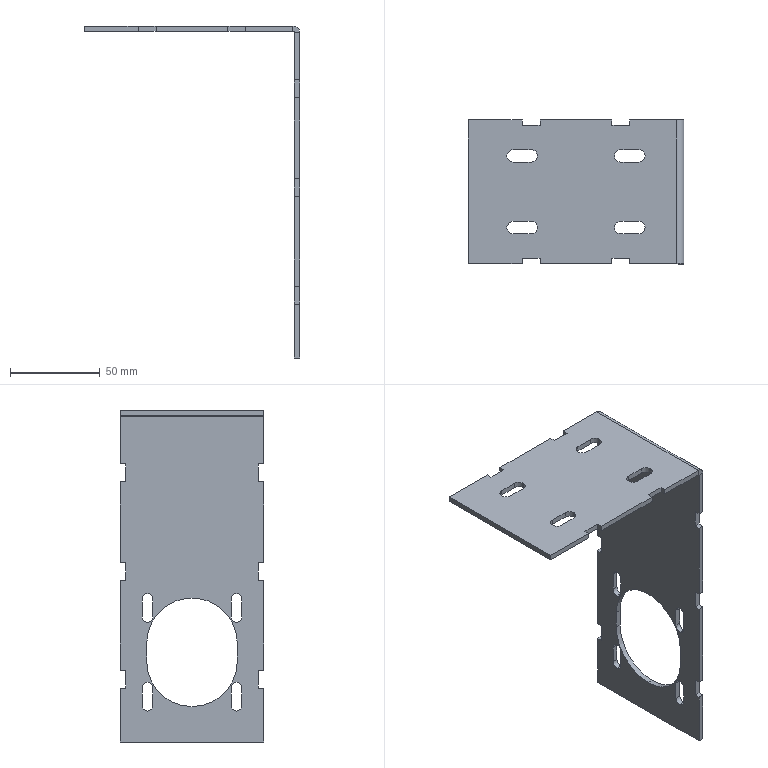Part | 1 solid | 99 faces | box 120 x 80 x 185 mm | volume 61465 mm3 | plane 70 | cylinder 29 | commonest cylinder face diameters 6 x12 7 x12 50.5 x3 1.473 x1 7.473 x1